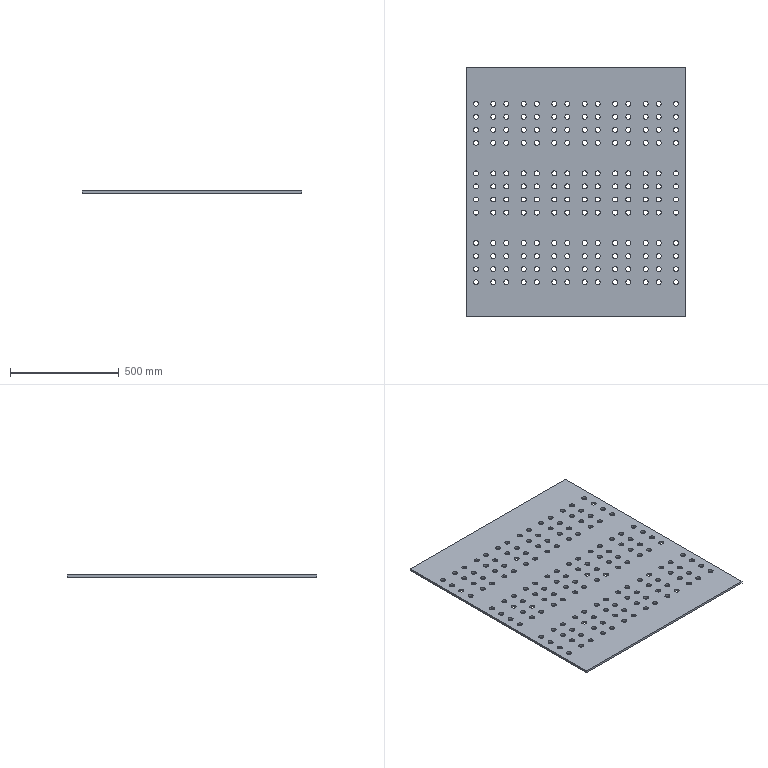Part | STEP file | 750038310 | 1 solid | 342 faces | box 1009 x 1149 x 10 mm | volume 10895411 mm3 | cylinder 336 | plane 6 | commonest cylinder face diameters 23 x336